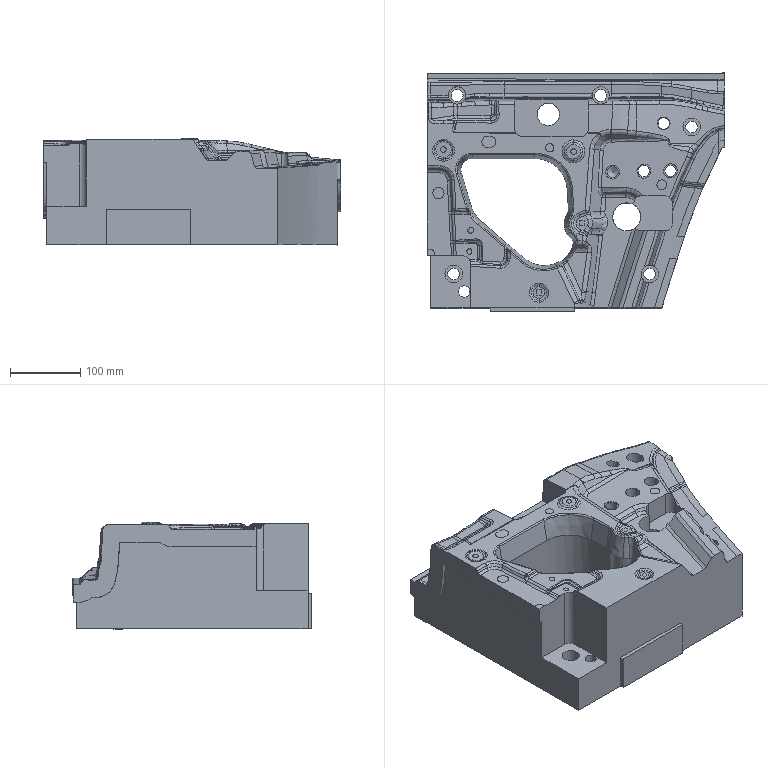Part | NX | features solid 2 | 1 solid | 491 faces | box 425 x 341.431 x 152.436 mm | volume 12844340 mm3 | spline 428 | plane 32 | cylinder 30 | cone 1 | commonest cylinder face diameters 20 x10 16 x5 17 x5 25 x5 23 x2 18 x1